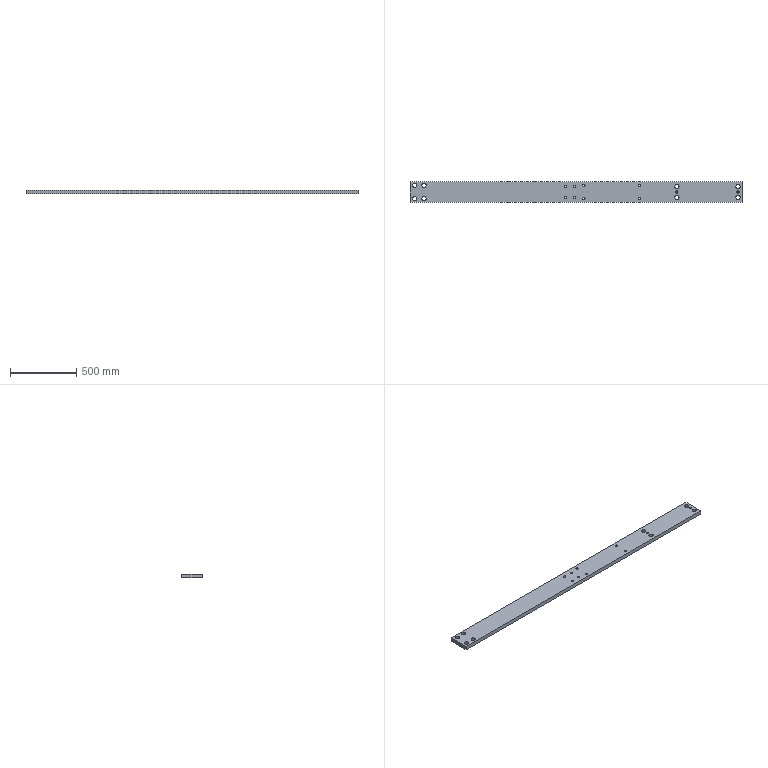Part | NX | features BREP 1 | 1 solid | 42 faces | box 2499 x 158 x 30 mm | volume 11579104 mm3 | cylinder 36 | plane 6 | commonest cylinder face diameters 18 x16 32 x16 16 x4
STEP:
#1=CARTESIAN_POINT('',(-1230.5,-50.,-15.));
#2=VERTEX_POINT('',#1);
#3=CARTESIAN_POINT('',(-1198.5,-50.,-15.));
#4=VERTEX_POINT('',#3);
#5=CARTESIAN_POINT('',(-1214.5,-50.,-15.));
#6=DIRECTION('',(0.,0.,1.));
#7=DIRECTION('',(-1.,0.,0.));
#8=AXIS2_PLACEMENT_3D('',#5,#6,#7);
#9=CIRCLE('',#8,16.);
#10=EDGE_CURVE('',#2,#4,#9,.T.);
#11=ORIENTED_EDGE('',*,*,#10,.F.);
#12=CARTESIAN_POINT('',(-1230.5,-50.,15.));
#13=VERTEX_POINT('',#12);
#14=CARTESIAN_POINT('',(-1230.5,-50.,-15.));
#15=DIRECTION('',(0.,0.,1.));
#16=VECTOR('',#15,1000.);
#17=LINE('',#14,#16);
#18=EDGE_CURVE('',#2,#13,#17,.T.);
#19=ORIENTED_EDGE('',*,*,#18,.T.);
#20=CARTESIAN_POINT('',(-1198.5,-50.,15.));
#21=VERTEX_POINT('',#20);
#22=CARTESIAN_POINT('',(-1214.5,-50.,15.));
#23=DIRECTION('',(0.,0.,1.));
#24=DIRECTION('',(-1.,0.,0.));
#25=AXIS2_PLACEMENT_3D('',#22,#23,#24);
#26=CIRCLE('',#25,16.);
#27=EDGE_CURVE('',#13,#21,#26,.T.);
#28=ORIENTED_EDGE('',*,*,#27,.T.);
#29=CARTESIAN_POINT('',(-1198.5,-50.,-15.));
#30=DIRECTION('',(0.,0.,1.));
#31=VECTOR('',#30,1000.);
#32=LINE('',#29,#31);
#33=EDGE_CURVE('',#4,#21,#32,.T.);
#34=ORIENTED_EDGE('',*,*,#33,.F.);
#35=EDGE_LOOP('',(#11,#19,#28,#34));
#36=FACE_BOUND('',#35,.T.);
#37=CARTESIAN_POINT('',(-1214.5,-50.,-15.));
#38=DIRECTION('',(0.,0.,1.));
#39=DIRECTION('',(-1.,0.,0.));
#40=AXIS2_PLACEMENT_3D('',#37,#38,#39);
#41=CYLINDRICAL_SURFACE('',#40,16.);
#42=ADVANCED_FACE('',(#36),#41,.F.);
#43=CARTESIAN_POINT('',(-1160.5,-50.,-15.));
#44=VERTEX_POINT('',#43);
#45=CARTESIAN_POINT('',(-1128.5,-50.,-15.));
#46=VERTEX_POINT('',#45);
#47=CARTESIAN_POINT('',(-1144.5,-50.,-15.));
#48=DIRECTION('',(0.,0.,1.));
#49=DIRECTION('',(-1.,0.,0.));
#50=AXIS2_PLACEMENT_3D('',#47,#48,#49);
#51=CIRCLE('',#50,16.);
#52=EDGE_CURVE('',#44,#46,#51,.T.);
#53=ORIENTED_EDGE('',*,*,#52,.F.);
#54=CARTESIAN_POINT('',(-1160.5,-50.,15.));
#55=VERTEX_POINT('',#54);
#56=CARTESIAN_POINT('',(-1160.5,-50.,-15.));
#57=DIRECTION('',(0.,0.,1.));
#58=VECTOR('',#57,1000.);
#59=LINE('',#56,#58);
#60=EDGE_CURVE('',#44,#55,#59,.T.);
#61=ORIENTED_EDGE('',*,*,#60,.T.);
#62=CARTESIAN_POINT('',(-1128.5,-50.,15.));
#63=VERTEX_POINT('',#62);
#64=CARTESIAN_POINT('',(-1144.5,-50.,15.));
#65=DIRECTION('',(0.,0.,1.));
#66=DIRECTION('',(-1.,0.,0.));
#67=AXIS2_PLACEMENT_3D('',#64,#65,#66);
#68=CIRCLE('',#67,16.);
#69=EDGE_CURVE('',#55,#63,#68,.T.);
#70=ORIENTED_EDGE('',*,*,#69,.T.);
#71=CARTESIAN_POINT('',(-1128.5,-50.,-15.));
#72=DIRECTION('',(0.,0.,1.));
#73=VECTOR('',#72,1000.);
#74=LINE('',#71,#73);
#75=EDGE_CURVE('',#46,#63,#74,.T.);
#76=ORIENTED_EDGE('',*,*,#75,.F.);
#77=EDGE_LOOP('',(#53,#61,#70,#76));
#78=FACE_BOUND('',#77,.T.);
#79=CARTESIAN_POINT('',(-1144.5,-50.,-15.));
#80=DIRECTION('',(0.,0.,1.));
#81=DIRECTION('',(-1.,0.,0.));
#82=AXIS2_PLACEMENT_3D('',#79,#80,#81);
#83=CYLINDRICAL_SURFACE('',#82,16.);
#84=ADVANCED_FACE('',(#78),#83,.F.);
#85=CARTESIAN_POINT('',(-1160.5,50.,-15.));
#86=VERTEX_POINT('',#85);
#87=CARTESIAN_POINT('',(-1128.5,50.,-15.));
#88=VERTEX_POINT('',#87);
#89=CARTESIAN_POINT('',(-1144.5,50.,-15.));
#90=DIRECTION('',(0.,0.,1.));
#91=DIRECTION('',(1.,0.,0.));
#92=AXIS2_PLACEMENT_3D('',#89,#90,#91);
#93=CIRCLE('',#92,16.);
#94=EDGE_CURVE('',#86,#88,#93,.T.);
#95=ORIENTED_EDGE('',*,*,#94,.F.);
#96=CARTESIAN_POINT('',(-1160.5,50.,15.));
#97=VERTEX_POINT('',#96);
#98=CARTESIAN_POINT('',(-1160.5,50.,-15.));
#99=DIRECTION('',(0.,0.,1.));
#100=VECTOR('',#99,1000.);
#101=LINE('',#98,#100);
#102=EDGE_CURVE('',#86,#97,#101,.T.);
#103=ORIENTED_EDGE('',*,*,#102,.T.);
#104=CARTESIAN_POINT('',(-1128.5,50.,15.));
#105=VERTEX_POINT('',#104);
#106=CARTESIAN_POINT('',(-1144.5,50.,15.));
#107=DIRECTION('',(0.,0.,1.));
#108=DIRECTION('',(1.,0.,0.));
#109=AXIS2_PLACEMENT_3D('',#106,#107,#108);
#110=CIRCLE('',#109,16.);
#111=EDGE_CURVE('',#97,#105,#110,.T.);
#112=ORIENTED_EDGE('',*,*,#111,.T.);
#113=CARTESIAN_POINT('',(-1128.5,50.,-15.));
#114=DIRECTION('',(0.,0.,1.));
#115=VECTOR('',#114,1000.);
#116=LINE('',#113,#115);
#117=EDGE_CURVE('',#88,#105,#116,.T.);
#118=ORIENTED_EDGE('',*,*,#117,.F.);
#119=EDGE_LOOP('',(#95,#103,#112,#118));
#120=FACE_BOUND('',#119,.T.);
#121=CARTESIAN_POINT('',(-1144.5,50.,-15.));
#122=DIRECTION('',(0.,0.,1.));
#123=DIRECTION('',(-1.,0.,0.));
#124=AXIS2_PLACEMENT_3D('',#121,#122,#123);
#125=CYLINDRICAL_SURFACE('',#124,16.);
#126=ADVANCED_FACE('',(#120),#125,.F.);
#127=CARTESIAN_POINT('',(-1230.5,50.,-15.));
#128=VERTEX_POINT('',#127);
#129=CARTESIAN_POINT('',(-1198.5,50.,-15.));
#130=VERTEX_POINT('',#129);
#131=CARTESIAN_POINT('',(-1214.5,50.,-15.));
#132=DIRECTION('',(0.,0.,1.));
#133=DIRECTION('',(1.,0.,0.));
#134=AXIS2_PLACEMENT_3D('',#131,#132,#133);
#135=CIRCLE('',#134,16.);
#136=EDGE_CURVE('',#128,#130,#135,.T.);
#137=ORIENTED_EDGE('',*,*,#136,.F.);
#138=CARTESIAN_POINT('',(-1230.5,50.,15.));
#139=VERTEX_POINT('',#138);
#140=CARTESIAN_POINT('',(-1230.5,50.,-15.));
#141=DIRECTION('',(0.,0.,1.));
#142=VECTOR('',#141,1000.);
#143=LINE('',#140,#142);
#144=EDGE_CURVE('',#128,#139,#143,.T.);
#145=ORIENTED_EDGE('',*,*,#144,.T.);
#146=CARTESIAN_POINT('',(-1198.5,50.,15.));
#147=VERTEX_POINT('',#146);
#148=CARTESIAN_POINT('',(-1214.5,50.,15.));
#149=DIRECTION('',(0.,0.,1.));
#150=DIRECTION('',(1.,0.,0.));
#151=AXIS2_PLACEMENT_3D('',#148,#149,#150);
#152=CIRCLE('',#151,16.);
#153=EDGE_CURVE('',#139,#147,#152,.T.);
#154=ORIENTED_EDGE('',*,*,#153,.T.);
#155=CARTESIAN_POINT('',(-1198.5,50.,-15.));
#156=DIRECTION('',(0.,0.,1.));
#157=VECTOR('',#156,1000.);
#158=LINE('',#155,#157);
#159=EDGE_CURVE('',#130,#147,#158,.T.);
#160=ORIENTED_EDGE('',*,*,#159,.F.);
#161=EDGE_LOOP('',(#137,#145,#154,#160));
#162=FACE_BOUND('',#161,.T.);
#163=CARTESIAN_POINT('',(-1214.5,50.,-15.));
#164=DIRECTION('',(0.,0.,1.));
#165=DIRECTION('',(-1.,0.,0.));
#166=AXIS2_PLACEMENT_3D('',#163,#164,#165);
#167=CYLINDRICAL_SURFACE('',#166,16.);
#168=ADVANCED_FACE('',(#162),#167,.F.);
#169=CARTESIAN_POINT('',(-89.5,-40.,-15.));
#170=VERTEX_POINT('',#169);
#171=CARTESIAN_POINT('',(-71.5,-40.,-15.));
#172=VERTEX_POINT('',#171);
#173=CARTESIAN_POINT('',(-80.5,-40.,-15.));
#174=DIRECTION('',(0.,0.,1.));
#175=DIRECTION('',(1.,0.,0.));
#176=AXIS2_PLACEMENT_3D('',#173,#174,#175);
#177=CIRCLE('',#176,9.);
#178=EDGE_CURVE('',#170,#172,#177,.T.);
#179=ORIENTED_EDGE('',*,*,#178,.F.);
#180=CARTESIAN_POINT('',(-89.5,-40.,15.));
#181=VERTEX_POINT('',#180);
#182=CARTESIAN_POINT('',(-89.5,-40.,-15.));
#183=DIRECTION('',(0.,0.,1.));
#184=VECTOR('',#183,1000.);
#185=LINE('',#182,#184);
#186=EDGE_CURVE('',#170,#181,#185,.T.);
#187=ORIENTED_EDGE('',*,*,#186,.T.);
#188=CARTESIAN_POINT('',(-71.5,-40.,15.));
#189=VERTEX_POINT('',#188);
#190=CARTESIAN_POINT('',(-80.5,-40.,15.));
#191=DIRECTION('',(0.,0.,1.));
#192=DIRECTION('',(1.,0.,0.));
#193=AXIS2_PLACEMENT_3D('',#190,#191,#192);
#194=CIRCLE('',#193,9.);
#195=EDGE_CURVE('',#181,#189,#194,.T.);
#196=ORIENTED_EDGE('',*,*,#195,.T.);
#197=CARTESIAN_POINT('',(-71.5,-40.,-15.));
#198=DIRECTION('',(0.,0.,1.));
#199=VECTOR('',#198,1000.);
#200=LINE('',#197,#199);
#201=EDGE_CURVE('',#172,#189,#200,.T.);
#202=ORIENTED_EDGE('',*,*,#201,.F.);
#203=EDGE_LOOP('',(#179,#187,#196,#202));
#204=FACE_BOUND('',#203,.T.);
#205=CARTESIAN_POINT('',(-80.5,-40.,-15.));
#206=DIRECTION('',(0.,0.,1.));
#207=DIRECTION('',(-1.,0.,0.));
#208=AXIS2_PLACEMENT_3D('',#205,#206,#207);
#209=CYLINDRICAL_SURFACE('',#208,9.);
#210=ADVANCED_FACE('',(#204),#209,.F.);
#211=CARTESIAN_POINT('',(-19.5,-40.,-15.));
#212=VERTEX_POINT('',#211);
#213=CARTESIAN_POINT('',(-1.5,-40.,-15.));
#214=VERTEX_POINT('',#213);
#215=CARTESIAN_POINT('',(-10.5,-40.,-15.));
#216=DIRECTION('',(0.,0.,1.));
#217=DIRECTION('',(1.,0.,0.));
#218=AXIS2_PLACEMENT_3D('',#215,#216,#217);
#219=CIRCLE('',#218,9.);
#220=EDGE_CURVE('',#212,#214,#219,.T.);
#221=ORIENTED_EDGE('',*,*,#220,.F.);
#222=CARTESIAN_POINT('',(-19.5,-40.,15.));
#223=VERTEX_POINT('',#222);
#224=CARTESIAN_POINT('',(-19.5,-40.,-15.));
#225=DIRECTION('',(0.,0.,1.));
#226=VECTOR('',#225,1000.);
#227=LINE('',#224,#226);
#228=EDGE_CURVE('',#212,#223,#227,.T.);
#229=ORIENTED_EDGE('',*,*,#228,.T.);
#230=CARTESIAN_POINT('',(-1.5,-40.,15.));
#231=VERTEX_POINT('',#230);
#232=CARTESIAN_POINT('',(-10.5,-40.,15.));
#233=DIRECTION('',(0.,0.,1.));
#234=DIRECTION('',(1.,0.,0.));
#235=AXIS2_PLACEMENT_3D('',#232,#233,#234);
#236=CIRCLE('',#235,9.);
#237=EDGE_CURVE('',#223,#231,#236,.T.);
#238=ORIENTED_EDGE('',*,*,#237,.T.);
#239=CARTESIAN_POINT('',(-1.5,-40.,-15.));
#240=DIRECTION('',(0.,0.,1.));
#241=VECTOR('',#240,1000.);
#242=LINE('',#239,#241);
#243=EDGE_CURVE('',#214,#231,#242,.T.);
#244=ORIENTED_EDGE('',*,*,#243,.F.);
#245=EDGE_LOOP('',(#221,#229,#238,#244));
#246=FACE_BOUND('',#245,.T.);
#247=CARTESIAN_POINT('',(-10.5,-40.,-15.));
#248=DIRECTION('',(0.,0.,1.));
#249=DIRECTION('',(-1.,0.,0.));
#250=AXIS2_PLACEMENT_3D('',#247,#248,#249);
#251=CYLINDRICAL_SURFACE('',#250,9.);
#252=ADVANCED_FACE('',(#246),#251,.F.);
#253=CARTESIAN_POINT('',(-89.5,40.,-15.));
#254=VERTEX_POINT('',#253);
#255=CARTESIAN_POINT('',(-71.5,40.,-15.));
#256=VERTEX_POINT('',#255);
#257=CARTESIAN_POINT('',(-80.5,40.,-15.));
#258=DIRECTION('',(0.,0.,1.));
#259=DIRECTION('',(1.,0.,0.));
#260=AXIS2_PLACEMENT_3D('',#257,#258,#259);
#261=CIRCLE('',#260,9.);
#262=EDGE_CURVE('',#254,#256,#261,.T.);
#263=ORIENTED_EDGE('',*,*,#262,.F.);
#264=CARTESIAN_POINT('',(-89.5,40.,15.));
#265=VERTEX_POINT('',#264);
#266=CARTESIAN_POINT('',(-89.5,40.,-15.));
#267=DIRECTION('',(0.,0.,1.));
#268=VECTOR('',#267,1000.);
#269=LINE('',#266,#268);
#270=EDGE_CURVE('',#254,#265,#269,.T.);
#271=ORIENTED_EDGE('',*,*,#270,.T.);
#272=CARTESIAN_POINT('',(-71.5,40.,15.));
#273=VERTEX_POINT('',#272);
#274=CARTESIAN_POINT('',(-80.5,40.,15.));
#275=DIRECTION('',(0.,0.,1.));
#276=DIRECTION('',(1.,0.,0.));
#277=AXIS2_PLACEMENT_3D('',#274,#275,#276);
#278=CIRCLE('',#277,9.);
#279=EDGE_CURVE('',#265,#273,#278,.T.);
#280=ORIENTED_EDGE('',*,*,#279,.T.);
#281=CARTESIAN_POINT('',(-71.5,40.,-15.));
#282=DIRECTION('',(0.,0.,1.));
#283=VECTOR('',#282,1000.);
#284=LINE('',#281,#283);
#285=EDGE_CURVE('',#256,#273,#284,.T.);
#286=ORIENTED_EDGE('',*,*,#285,.F.);
#287=EDGE_LOOP('',(#263,#271,#280,#286));
#288=FACE_BOUND('',#287,.T.);
#289=CARTESIAN_POINT('',(-80.5,40.,-15.));
#290=DIRECTION('',(0.,0.,1.));
#291=DIRECTION('',(-1.,0.,0.));
#292=AXIS2_PLACEMENT_3D('',#289,#290,#291);
#293=CYLINDRICAL_SURFACE('',#292,9.);
#294=ADVANCED_FACE('',(#288),#293,.F.);
#295=CARTESIAN_POINT('',(-19.5,40.,-15.));
#296=VERTEX_POINT('',#295);
#297=CARTESIAN_POINT('',(-1.5,40.,-15.));
#298=VERTEX_POINT('',#297);
#299=CARTESIAN_POINT('',(-10.5,40.,-15.));
#300=DIRECTION('',(0.,0.,1.));
#301=DIRECTION('',(1.,0.,0.));
#302=AXIS2_PLACEMENT_3D('',#299,#300,#301);
#303=CIRCLE('',#302,9.);
#304=EDGE_CURVE('',#296,#298,#303,.T.);
#305=ORIENTED_EDGE('',*,*,#304,.F.);
#306=CARTESIAN_POINT('',(-19.5,40.,15.));
#307=VERTEX_POINT('',#306);
#308=CARTESIAN_POINT('',(-19.5,40.,-15.));
#309=DIRECTION('',(0.,0.,1.));
#310=VECTOR('',#309,1000.);
#311=LINE('',#308,#310);
#312=EDGE_CURVE('',#296,#307,#311,.T.);
#313=ORIENTED_EDGE('',*,*,#312,.T.);
#314=CARTESIAN_POINT('',(-1.5,40.,15.));
#315=VERTEX_POINT('',#314);
#316=CARTESIAN_POINT('',(-10.5,40.,15.));
#317=DIRECTION('',(0.,0.,1.));
#318=DIRECTION('',(1.,0.,0.));
#319=AXIS2_PLACEMENT_3D('',#316,#317,#318);
#320=CIRCLE('',#319,9.);
#321=EDGE_CURVE('',#307,#315,#320,.T.);
#322=ORIENTED_EDGE('',*,*,#321,.T.);
#323=CARTESIAN_POINT('',(-1.5,40.,-15.));
#324=DIRECTION('',(0.,0.,1.));
#325=VECTOR('',#324,1000.);
#326=LINE('',#323,#325);
#327=EDGE_CURVE('',#298,#315,#326,.T.);
#328=ORIENTED_EDGE('',*,*,#327,.F.);
#329=EDGE_LOOP('',(#305,#313,#322,#328));
#330=FACE_BOUND('',#329,.T.);
#331=CARTESIAN_POINT('',(-10.5,40.,-15.));
#332=DIRECTION('',(0.,0.,1.));
#333=DIRECTION('',(-1.,0.,0.));
#334=AXIS2_PLACEMENT_3D('',#331,#332,#333);
#335=CYLINDRICAL_SURFACE('',#334,9.);
#336=ADVANCED_FACE('',(#330),#335,.F.);
#337=CARTESIAN_POINT('',(50.5,-50.,-15.));
#338=VERTEX_POINT('',#337);
#339=CARTESIAN_POINT('',(68.5,-50.,-15.));
#340=VERTEX_POINT('',#339);
#341=CARTESIAN_POINT('',(59.5,-50.,-15.));
#342=DIRECTION('',(0.,0.,1.));
#343=DIRECTION('',(1.,0.,0.));
#344=AXIS2_PLACEMENT_3D('',#341,#342,#343);
#345=CIRCLE('',#344,9.);
#346=EDGE_CURVE('',#338,#340,#345,.T.);
#347=ORIENTED_EDGE('',*,*,#346,.F.);
#348=CARTESIAN_POINT('',(50.5,-50.,15.));
#349=VERTEX_POINT('',#348);
#350=CARTESIAN_POINT('',(50.5,-50.,-15.));
#351=DIRECTION('',(0.,0.,1.));
#352=VECTOR('',#351,1000.);
#353=LINE('',#350,#352);
#354=EDGE_CURVE('',#338,#349,#353,.T.);
#355=ORIENTED_EDGE('',*,*,#354,.T.);
#356=CARTESIAN_POINT('',(68.5,-50.,15.));
#357=VERTEX_POINT('',#356);
#358=CARTESIAN_POINT('',(59.5,-50.,15.));
#359=DIRECTION('',(0.,0.,1.));
#360=DIRECTION('',(1.,0.,0.));
#361=AXIS2_PLACEMENT_3D('',#358,#359,#360);
#362=CIRCLE('',#361,9.);
#363=EDGE_CURVE('',#349,#357,#362,.T.);
#364=ORIENTED_EDGE('',*,*,#363,.T.);
#365=CARTESIAN_POINT('',(68.5,-50.,-15.));
#366=DIRECTION('',(0.,0.,1.));
#367=VECTOR('',#366,1000.);
#368=LINE('',#365,#367);
#369=EDGE_CURVE('',#340,#357,#368,.T.);
#370=ORIENTED_EDGE('',*,*,#369,.F.);
#371=EDGE_LOOP('',(#347,#355,#364,#370));
#372=FACE_BOUND('',#371,.T.);
#373=CARTESIAN_POINT('',(59.5,-50.,-15.));
#374=DIRECTION('',(0.,0.,1.));
#375=DIRECTION('',(-1.,0.,0.));
#376=AXIS2_PLACEMENT_3D('',#373,#374,#375);
#377=CYLINDRICAL_SURFACE('',#376,9.);
#378=ADVANCED_FACE('',(#372),#377,.F.);
#379=CARTESIAN_POINT('',(50.5,50.,-15.));
#380=VERTEX_POINT('',#379);
#381=CARTESIAN_POINT('',(68.5,50.,-15.));
#382=VERTEX_POINT('',#381);
#383=CARTESIAN_POINT('',(59.5,50.,-15.));
#384=DIRECTION('',(0.,0.,1.));
#385=DIRECTION('',(-1.,0.,0.));
#386=AXIS2_PLACEMENT_3D('',#383,#384,#385);
#387=CIRCLE('',#386,9.);
#388=EDGE_CURVE('',#380,#382,#387,.T.);
#389=ORIENTED_EDGE('',*,*,#388,.F.);
#390=CARTESIAN_POINT('',(50.5,50.,15.));
#391=VERTEX_POINT('',#390);
#392=CARTESIAN_POINT('',(50.5,50.,-15.));
#393=DIRECTION('',(0.,0.,1.));
#394=VECTOR('',#393,1000.);
#395=LINE('',#392,#394);
#396=EDGE_CURVE('',#380,#391,#395,.T.);
#397=ORIENTED_EDGE('',*,*,#396,.T.);
#398=CARTESIAN_POINT('',(68.5,50.,15.));
#399=VERTEX_POINT('',#398);
#400=CARTESIAN_POINT('',(59.5,50.,15.));
#401=DIRECTION('',(0.,0.,1.));
#402=DIRECTION('',(-1.,0.,0.));
#403=AXIS2_PLACEMENT_3D('',#400,#401,#402);
#404=CIRCLE('',#403,9.);
#405=EDGE_CURVE('',#391,#399,#404,.T.);
#406=ORIENTED_EDGE('',*,*,#405,.T.);
#407=CARTESIAN_POINT('',(68.5,50.,-15.));
#408=DIRECTION('',(0.,0.,1.));
#409=VECTOR('',#408,1000.);
#410=LINE('',#407,#409);
#411=EDGE_CURVE('',#382,#399,#410,.T.);
#412=ORIENTED_EDGE('',*,*,#411,.F.);
#413=EDGE_LOOP('',(#389,#397,#406,#412));
#414=FACE_BOUND('',#413,.T.);
#415=CARTESIAN_POINT('',(59.5,50.,-15.));
#416=DIRECTION('',(0.,0.,1.));
#417=DIRECTION('',(-1.,0.,0.));
#418=AXIS2_PLACEMENT_3D('',#415,#416,#417);
#419=CYLINDRICAL_SURFACE('',#418,9.);
#420=ADVANCED_FACE('',(#414),#419,.F.);
#421=CARTESIAN_POINT('',(470.5,-50.,-15.));
#422=VERTEX_POINT('',#421);
#423=CARTESIAN_POINT('',(488.5,-50.,-15.));
#424=VERTEX_POINT('',#423);
#425=CARTESIAN_POINT('',(479.5,-50.,-15.));
#426=DIRECTION('',(0.,0.,1.));
#427=DIRECTION('',(-1.,0.,0.));
#428=AXIS2_PLACEMENT_3D('',#425,#426,#427);
#429=CIRCLE('',#428,9.);
#430=EDGE_CURVE('',#422,#424,#429,.T.);
#431=ORIENTED_EDGE('',*,*,#430,.F.);
#432=CARTESIAN_POINT('',(470.5,-50.,15.));
#433=VERTEX_POINT('',#432);
#434=CARTESIAN_POINT('',(470.5,-50.,-15.));
#435=DIRECTION('',(0.,0.,1.));
#436=VECTOR('',#435,1000.);
#437=LINE('',#434,#436);
#438=EDGE_CURVE('',#422,#433,#437,.T.);
#439=ORIENTED_EDGE('',*,*,#438,.T.);
#440=CARTESIAN_POINT('',(488.5,-50.,15.));
#441=VERTEX_POINT('',#440);
#442=CARTESIAN_POINT('',(479.5,-50.,15.));
#443=DIRECTION('',(0.,0.,1.));
#444=DIRECTION('',(-1.,0.,0.));
#445=AXIS2_PLACEMENT_3D('',#442,#443,#444);
#446=CIRCLE('',#445,9.);
#447=EDGE_CURVE('',#433,#441,#446,.T.);
#448=ORIENTED_EDGE('',*,*,#447,.T.);
#449=CARTESIAN_POINT('',(488.5,-50.,-15.));
#450=DIRECTION('',(0.,0.,1.));
#451=VECTOR('',#450,1000.);
#452=LINE('',#449,#451);
#453=EDGE_CURVE('',#424,#441,#452,.T.);
#454=ORIENTED_EDGE('',*,*,#453,.F.);
#455=EDGE_LOOP('',(#431,#439,#448,#454));
#456=FACE_BOUND('',#455,.T.);
#457=CARTESIAN_POINT('',(479.5,-50.,-15.));
#458=DIRECTION('',(0.,0.,1.));
#459=DIRECTION('',(-1.,0.,0.));
#460=AXIS2_PLACEMENT_3D('',#457,#458,#459);
#461=CYLINDRICAL_SURFACE('',#460,9.);
#462=ADVANCED_FACE('',(#456),#461,.F.);
#463=CARTESIAN_POINT('',(470.5,50.,-15.));
#464=VERTEX_POINT('',#463);
#465=CARTESIAN_POINT('',(488.5,50.,-15.));
#466=VERTEX_POINT('',#465);
#467=CARTESIAN_POINT('',(479.5,50.,-15.));
#468=DIRECTION('',(0.,0.,1.));
#469=DIRECTION('',(1.,0.,0.));
#470=AXIS2_PLACEMENT_3D('',#467,#468,#469);
#471=CIRCLE('',#470,9.);
#472=EDGE_CURVE('',#464,#466,#471,.T.);
#473=ORIENTED_EDGE('',*,*,#472,.F.);
#474=CARTESIAN_POINT('',(470.5,50.,15.));
#475=VERTEX_POINT('',#474);
#476=CARTESIAN_POINT('',(470.5,50.,-15.));
#477=DIRECTION('',(0.,0.,1.));
#478=VECTOR('',#477,1000.);
#479=LINE('',#476,#478);
#480=EDGE_CURVE('',#464,#475,#479,.T.);
#481=ORIENTED_EDGE('',*,*,#480,.T.);
#482=CARTESIAN_POINT('',(488.5,50.,15.));
#483=VERTEX_POINT('',#482);
#484=CARTESIAN_POINT('',(479.5,50.,15.));
#485=DIRECTION('',(0.,0.,1.));
#486=DIRECTION('',(1.,0.,0.));
#487=AXIS2_PLACEMENT_3D('',#484,#485,#486);
#488=CIRCLE('',#487,9.);
#489=EDGE_CURVE('',#475,#483,#488,.T.);
#490=ORIENTED_EDGE('',*,*,#489,.T.);
#491=CARTESIAN_POINT('',(488.5,50.,-15.));
#492=DIRECTION('',(0.,0.,1.));
#493=VECTOR('',#492,1000.);
#494=LINE('',#491,#493);
#495=EDGE_CURVE('',#466,#483,#494,.T.);
#496=ORIENTED_EDGE('',*,*,#495,.F.);
#497=EDGE_LOOP('',(#473,#481,#490,#496));
#498=FACE_BOUND('',#497,.T.);
#499=CARTESIAN_POINT('',(479.5,50.,-15.));
#500=DIRECTION('',(0.,0.,1.));
#501=DIRECTION('',(-1.,0.,0.));
#502=AXIS2_PLACEMENT_3D('',#499,#500,#501);
#503=CYLINDRICAL_SURFACE('',#502,9.);
#504=ADVANCED_FACE('',(#498),#503,.F.);
#505=CARTESIAN_POINT('',(743.5,40.,-15.));
#506=VERTEX_POINT('',#505);
#507=CARTESIAN_POINT('',(775.5,40.,-15.));
#508=VERTEX_POINT('',#507);
#509=CARTESIAN_POINT('',(759.5,40.,-15.));
#510=DIRECTION('',(0.,0.,1.));
#511=DIRECTION('',(-1.,0.,0.));
#512=AXIS2_PLACEMENT_3D('',#509,#510,#511);
#513=CIRCLE('',#512,16.);
#514=EDGE_CURVE('',#506,#508,#513,.T.);
#515=ORIENTED_EDGE('',*,*,#514,.F.);
#516=CARTESIAN_POINT('',(743.5,40.,15.));
#517=VERTEX_POINT('',#516);
#518=CARTESIAN_POINT('',(743.5,40.,-15.));
#519=DIRECTION('',(0.,0.,1.));
#520=VECTOR('',#519,1000.);
#521=LINE('',#518,#520);
#522=EDGE_CURVE('',#506,#517,#521,.T.);
#523=ORIENTED_EDGE('',*,*,#522,.T.);
#524=CARTESIAN_POINT('',(775.5,40.,15.));
#525=VERTEX_POINT('',#524);
#526=CARTESIAN_POINT('',(759.5,40.,15.));
#527=DIRECTION('',(0.,0.,1.));
#528=DIRECTION('',(-1.,0.,0.));
#529=AXIS2_PLACEMENT_3D('',#526,#527,#528);
#530=CIRCLE('',#529,16.);
#531=EDGE_CURVE('',#517,#525,#530,.T.);
#532=ORIENTED_EDGE('',*,*,#531,.T.);
#533=CARTESIAN_POINT('',(775.5,40.,-15.));
#534=DIRECTION('',(0.,0.,1.));
#535=VECTOR('',#534,1000.);
#536=LINE('',#533,#535);
#537=EDGE_CURVE('',#508,#525,#536,.T.);
#538=ORIENTED_EDGE('',*,*,#537,.F.);
#539=EDGE_LOOP('',(#515,#523,#532,#538));
#540=FACE_BOUND('',#539,.T.);
#541=CARTESIAN_POINT('',(759.5,40.,-15.));
#542=DIRECTION('',(0.,0.,1.));
#543=DIRECTION('',(-1.,0.,0.));
#544=AXIS2_PLACEMENT_3D('',#541,#542,#543);
#545=CYLINDRICAL_SURFACE('',#544,16.);
#546=ADVANCED_FACE('',(#540),#545,.F.);
#547=CARTESIAN_POINT('',(743.5,-40.,-15.));
#548=VERTEX_POINT('',#547);
#549=CARTESIAN_POINT('',(775.5,-40.,-15.));
#550=VERTEX_POINT('',#549);
#551=CARTESIAN_POINT('',(759.5,-40.,-15.));
#552=DIRECTION('',(0.,0.,1.));
#553=DIRECTION('',(1.,0.,0.));
#554=AXIS2_PLACEMENT_3D('',#551,#552,#553);
#555=CIRCLE('',#554,16.);
#556=EDGE_CURVE('',#548,#550,#555,.T.);
#557=ORIENTED_EDGE('',*,*,#556,.F.);
#558=CARTESIAN_POINT('',(743.5,-40.,15.));
#559=VERTEX_POINT('',#558);
#560=CARTESIAN_POINT('',(743.5,-40.,-15.));
#561=DIRECTION('',(0.,0.,1.));
#562=VECTOR('',#561,1000.);
#563=LINE('',#560,#562);
#564=EDGE_CURVE('',#548,#559,#563,.T.);
#565=ORIENTED_EDGE('',*,*,#564,.T.);
#566=CARTESIAN_POINT('',(775.5,-40.,15.));
#567=VERTEX_POINT('',#566);
#568=CARTESIAN_POINT('',(759.5,-40.,15.));
#569=DIRECTION('',(0.,0.,1.));
#570=DIRECTION('',(1.,0.,0.));
#571=AXIS2_PLACEMENT_3D('',#568,#569,#570);
#572=CIRCLE('',#571,16.);
#573=EDGE_CURVE('',#559,#567,#572,.T.);
#574=ORIENTED_EDGE('',*,*,#573,.T.);
#575=CARTESIAN_POINT('',(775.5,-40.,-15.));
#576=DIRECTION('',(0.,0.,1.));
#577=VECTOR('',#576,1000.);
#578=LINE('',#575,#577);
#579=EDGE_CURVE('',#550,#567,#578,.T.);
#580=ORIENTED_EDGE('',*,*,#579,.F.);
#581=EDGE_LOOP('',(#557,#565,#574,#580));
#582=FACE_BOUND('',#581,.T.);
#583=CARTESIAN_POINT('',(759.5,-40.,-15.));
#584=DIRECTION('',(0.,0.,1.));
#585=DIRECTION('',(-1.,0.,0.));
#586=AXIS2_PLACEMENT_3D('',#583,#584,#585);
#587=CYLINDRICAL_SURFACE('',#586,16.);
#588=ADVANCED_FACE('',(#582),#587,.F.);
#589=CARTESIAN_POINT('',(751.5,0.,-15.));
#590=VERTEX_POINT('',#589);
#591=CARTESIAN_POINT('',(767.5,0.,-15.));
#592=VERTEX_POINT('',#591);
#593=CARTESIAN_POINT('',(759.5,0.,-15.));
#594=DIRECTION('',(0.,0.,1.));
#595=DIRECTION('',(-1.,0.,0.));
#596=AXIS2_PLACEMENT_3D('',#593,#594,#595);
#597=CIRCLE('',#596,8.);
#598=EDGE_CURVE('',#590,#592,#597,.T.);
#599=ORIENTED_EDGE('',*,*,#598,.F.);
#600=CARTESIAN_POINT('',(751.5,0.,15.));
#601=VERTEX_POINT('',#600);
#602=CARTESIAN_POINT('',(751.5,0.,-15.));
#603=DIRECTION('',(0.,0.,1.));
#604=VECTOR('',#603,1000.);
#605=LINE('',#602,#604);
#606=EDGE_CURVE('',#590,#601,#605,.T.);
#607=ORIENTED_EDGE('',*,*,#606,.T.);
#608=CARTESIAN_POINT('',(767.5,0.,15.));
#609=VERTEX_POINT('',#608);
#610=CARTESIAN_POINT('',(759.5,0.,15.));
#611=DIRECTION('',(0.,0.,1.));
#612=DIRECTION('',(-1.,0.,0.));
#613=AXIS2_PLACEMENT_3D('',#610,#611,#612);
#614=CIRCLE('',#613,8.);
#615=EDGE_CURVE('',#601,#609,#614,.T.);
#616=ORIENTED_EDGE('',*,*,#615,.T.);
#617=CARTESIAN_POINT('',(767.5,0.,-15.));
#618=DIRECTION('',(0.,0.,1.));
#619=VECTOR('',#618,1000.);
#620=LINE('',#617,#619);
#621=EDGE_CURVE('',#592,#609,#620,.T.);
#622=ORIENTED_EDGE('',*,*,#621,.F.);
#623=EDGE_LOOP('',(#599,#607,#616,#622));
#624=FACE_BOUND('',#623,.T.);
#625=CARTESIAN_POINT('',(759.5,0.,-15.));
#626=DIRECTION('',(0.,0.,1.));
#627=DIRECTION('',(-1.,0.,0.));
#628=AXIS2_PLACEMENT_3D('',#625,#626,#627);
#629=CYLINDRICAL_SURFACE('',#628,8.);
#630=ADVANCED_FACE('',(#624),#629,.F.);
#631=CARTESIAN_POINT('',(1211.5,0.,-15.));
#632=VERTEX_POINT('',#631);
#633=CARTESIAN_POINT('',(1227.5,0.,-15.));
#634=VERTEX_POINT('',#633);
#635=CARTESIAN_POINT('',(1219.5,0.,-15.));
#636=DIRECTION('',(0.,0.,1.));
#637=DIRECTION('',(1.,0.,0.));
#638=AXIS2_PLACEMENT_3D('',#635,#636,#637);
#639=CIRCLE('',#638,8.);
#640=EDGE_CURVE('',#632,#634,#639,.T.);
#641=ORIENTED_EDGE('',*,*,#640,.F.);
#642=CARTESIAN_POINT('',(1211.5,0.,15.));
#643=VERTEX_POINT('',#642);
#644=CARTESIAN_POINT('',(1211.5,0.,-15.));
#645=DIRECTION('',(0.,0.,1.));
#646=VECTOR('',#645,1000.);
#647=LINE('',#644,#646);
#648=EDGE_CURVE('',#632,#643,#647,.T.);
#649=ORIENTED_EDGE('',*,*,#648,.T.);
#650=CARTESIAN_POINT('',(1227.5,0.,15.));
#651=VERTEX_POINT('',#650);
#652=CARTESIAN_POINT('',(1219.5,0.,15.));
#653=DIRECTION('',(0.,0.,1.));
#654=DIRECTION('',(1.,0.,0.));
#655=AXIS2_PLACEMENT_3D('',#652,#653,#654);
#656=CIRCLE('',#655,8.);
#657=EDGE_CURVE('',#643,#651,#656,.T.);
#658=ORIENTED_EDGE('',*,*,#657,.T.);
#659=CARTESIAN_POINT('',(1227.5,0.,-15.));
#660=DIRECTION('',(0.,0.,1.));
#661=VECTOR('',#660,1000.);
#662=LINE('',#659,#661);
#663=EDGE_CURVE('',#634,#651,#662,.T.);
#664=ORIENTED_EDGE('',*,*,#663,.F.);
#665=EDGE_LOOP('',(#641,#649,#658,#664));
#666=FACE_BOUND('',#665,.T.);
#667=CARTESIAN_POINT('',(1219.5,0.,-15.));
#668=DIRECTION('',(0.,0.,1.));
#669=DIRECTION('',(-1.,0.,0.));
#670=AXIS2_PLACEMENT_3D('',#667,#668,#669);
#671=CYLINDRICAL_SURFACE('',#670,8.);
#672=ADVANCED_FACE('',(#666),#671,.F.);
#673=CARTESIAN_POINT('',(1203.5,-40.,-15.));
#674=VERTEX_POINT('',#673);
#675=CARTESIAN_POINT('',(1235.5,-40.,-15.));
#676=VERTEX_POINT('',#675);
#677=CARTESIAN_POINT('',(1219.5,-40.,-15.));
#678=DIRECTION('',(0.,0.,1.));
#679=DIRECTION('',(-1.,0.,0.));
#680=AXIS2_PLACEMENT_3D('',#677,#678,#679);
#681=CIRCLE('',#680,16.);
#682=EDGE_CURVE('',#674,#676,#681,.T.);
#683=ORIENTED_EDGE('',*,*,#682,.F.);
#684=CARTESIAN_POINT('',(1203.5,-40.,15.));
#685=VERTEX_POINT('',#684);
#686=CARTESIAN_POINT('',(1203.5,-40.,-15.));
#687=DIRECTION('',(0.,0.,1.));
#688=VECTOR('',#687,1000.);
#689=LINE('',#686,#688);
#690=EDGE_CURVE('',#674,#685,#689,.T.);
#691=ORIENTED_EDGE('',*,*,#690,.T.);
#692=CARTESIAN_POINT('',(1235.5,-40.,15.));
#693=VERTEX_POINT('',#692);
#694=CARTESIAN_POINT('',(1219.5,-40.,15.));
#695=DIRECTION('',(0.,0.,1.));
#696=DIRECTION('',(-1.,0.,0.));
#697=AXIS2_PLACEMENT_3D('',#694,#695,#696);
#698=CIRCLE('',#697,16.);
#699=EDGE_CURVE('',#685,#693,#698,.T.);
#700=ORIENTED_EDGE('',*,*,#699,.T.);
#701=CARTESIAN_POINT('',(1235.5,-40.,-15.));
#702=DIRECTION('',(0.,0.,1.));
#703=VECTOR('',#702,1000.);
#704=LINE('',#701,#703);
#705=EDGE_CURVE('',#676,#693,#704,.T.);
#706=ORIENTED_EDGE('',*,*,#705,.F.);
#707=EDGE_LOOP('',(#683,#691,#700,#706));
#708=FACE_BOUND('',#707,.T.);
#709=CARTESIAN_POINT('',(1219.5,-40.,-15.));
#710=DIRECTION('',(0.,0.,1.));
#711=DIRECTION('',(-1.,0.,0.));
#712=AXIS2_PLACEMENT_3D('',#709,#710,#711);
#713=CYLINDRICAL_SURFACE('',#712,16.);
#714=ADVANCED_FACE('',(#708),#713,.F.);
#715=CARTESIAN_POINT('',(1203.5,40.,-15.));
#716=VERTEX_POINT('',#715);
#717=CARTESIAN_POINT('',(1235.5,40.,-15.));
#718=VERTEX_POINT('',#717);
#719=CARTESIAN_POINT('',(1219.5,40.,-15.));
#720=DIRECTION('',(0.,0.,1.));
#721=DIRECTION('',(1.,0.,0.));
#722=AXIS2_PLACEMENT_3D('',#719,#720,#721);
#723=CIRCLE('',#722,16.);
#724=EDGE_CURVE('',#716,#718,#723,.T.);
#725=ORIENTED_EDGE('',*,*,#724,.F.);
#726=CARTESIAN_POINT('',(1203.5,40.,15.));
#727=VERTEX_POINT('',#726);
#728=CARTESIAN_POINT('',(1203.5,40.,-15.));
#729=DIRECTION('',(0.,0.,1.));
#730=VECTOR('',#729,1000.);
#731=LINE('',#728,#730);
#732=EDGE_CURVE('',#716,#727,#731,.T.);
#733=ORIENTED_EDGE('',*,*,#732,.T.);
#734=CARTESIAN_POINT('',(1235.5,40.,15.));
#735=VERTEX_POINT('',#734);
#736=CARTESIAN_POINT('',(1219.5,40.,15.));
#737=DIRECTION('',(0.,0.,1.));
#738=DIRECTION('',(1.,0.,0.));
#739=AXIS2_PLACEMENT_3D('',#736,#737,#738);
#740=CIRCLE('',#739,16.);
#741=EDGE_CURVE('',#727,#735,#740,.T.);
#742=ORIENTED_EDGE('',*,*,#741,.T.);
#743=CARTESIAN_POINT('',(1235.5,40.,-15.));
#744=DIRECTION('',(0.,0.,1.));
#745=VECTOR('',#744,1000.);
#746=LINE('',#743,#745);
#747=EDGE_CURVE('',#718,#735,#746,.T.);
#748=ORIENTED_EDGE('',*,*,#747,.F.);
#749=EDGE_LOOP('',(#725,#733,#742,#748));
#750=FACE_BOUND('',#749,.T.);
#751=CARTESIAN_POINT('',(1219.5,40.,-15.));
#752=DIRECTION('',(0.,0.,1.));
#753=DIRECTION('',(-1.,0.,0.));
#754=AXIS2_PLACEMENT_3D('',#751,#752,#753);
#755=CYLINDRICAL_SURFACE('',#754,16.);
#756=ADVANCED_FACE('',(#750),#755,.F.);
#757=CARTESIAN_POINT('',(-1249.5,79.,-15.));
#758=VERTEX_POINT('',#757);
#759=CARTESIAN_POINT('',(-1249.5,-79.,-15.));
#760=VERTEX_POINT('',#759);
#761=CARTESIAN_POINT('',(-1249.5,79.,-15.));
#762=DIRECTION('',(0.,-1.,0.));
#763=VECTOR('',#762,1000.);
#764=LINE('',#761,#763);
#765=EDGE_CURVE('',#758,#760,#764,.T.);
#766=ORIENTED_EDGE('',*,*,#765,.T.);
#767=CARTESIAN_POINT('',(-1249.5,-79.,15.));
#768=VERTEX_POINT('',#767);
#769=CARTESIAN_POINT('',(-1249.5,-79.,15.));
#770=DIRECTION('',(0.,0.,-1.));
#771=VECTOR('',#770,1000.);
#772=LINE('',#769,#771);
#773=EDGE_CURVE('',#768,#760,#772,.T.);
#774=ORIENTED_EDGE('',*,*,#773,.F.);
#775=CARTESIAN_POINT('',(-1249.5,79.,15.));
#776=VERTEX_POINT('',#775);
#777=CARTESIAN_POINT('',(-1249.5,79.,15.));
#778=DIRECTION('',(0.,-1.,0.));
#779=VECTOR('',#778,1000.);
#780=LINE('',#777,#779);
#781=EDGE_CURVE('',#776,#768,#780,.T.);
#782=ORIENTED_EDGE('',*,*,#781,.F.);
#783=CARTESIAN_POINT('',(-1249.5,79.,15.));
#784=DIRECTION('',(0.,0.,-1.));
#785=VECTOR('',#784,1000.);
#786=LINE('',#783,#785);
#787=EDGE_CURVE('',#776,#758,#786,.T.);
#788=ORIENTED_EDGE('',*,*,#787,.T.);
#789=EDGE_LOOP('',(#766,#774,#782,#788));
#790=FACE_BOUND('',#789,.T.);
#791=CARTESIAN_POINT('',(-1249.5,79.,15.));
#792=DIRECTION('',(1.,0.,0.));
#793=DIRECTION('',(0.,0.,1.));
#794=AXIS2_PLACEMENT_3D('',#791,#792,#793);
#795=PLANE('',#794);
#796=ADVANCED_FACE('',(#790),#795,.F.);
#797=CARTESIAN_POINT('',(1249.5,-79.,-15.));
#798=VERTEX_POINT('',#797);
#799=CARTESIAN_POINT('',(-1249.5,-79.,-15.));
#800=DIRECTION('',(1.,0.,0.));
#801=VECTOR('',#800,1000.);
#802=LINE('',#799,#801);
#803=EDGE_CURVE('',#760,#798,#802,.T.);
#804=ORIENTED_EDGE('',*,*,#803,.T.);
#805=CARTESIAN_POINT('',(1249.5,-79.,15.));
#806=VERTEX_POINT('',#805);
#807=CARTESIAN_POINT('',(1249.5,-79.,15.));
#808=DIRECTION('',(0.,0.,-1.));
#809=VECTOR('',#808,1000.);
#810=LINE('',#807,#809);
#811=EDGE_CURVE('',#806,#798,#810,.T.);
#812=ORIENTED_EDGE('',*,*,#811,.F.);
#813=CARTESIAN_POINT('',(-1249.5,-79.,15.));
#814=DIRECTION('',(1.,0.,0.));
#815=VECTOR('',#814,1000.);
#816=LINE('',#813,#815);
#817=EDGE_CURVE('',#768,#806,#816,.T.);
#818=ORIENTED_EDGE('',*,*,#817,.F.);
#819=ORIENTED_EDGE('',*,*,#773,.T.);
#820=EDGE_LOOP('',(#804,#812,#818,#819));
#821=FACE_BOUND('',#820,.T.);
#822=CARTESIAN_POINT('',(-1249.5,-79.,15.));
#823=DIRECTION('',(0.,1.,0.));
#824=DIRECTION('',(0.,0.,-1.));
#825=AXIS2_PLACEMENT_3D('',#822,#823,#824);
#826=PLANE('',#825);
#827=ADVANCED_FACE('',(#821),#826,.F.);
#828=CARTESIAN_POINT('',(1249.5,79.,-15.));
#829=VERTEX_POINT('',#828);
#830=CARTESIAN_POINT('',(1249.5,79.,-15.));
#831=DIRECTION('',(0.,1.,0.));
#832=VECTOR('',#831,1000.);
#833=LINE('',#830,#832);
#834=EDGE_CURVE('',#798,#829,#833,.T.);
#835=ORIENTED_EDGE('',*,*,#834,.T.);
#836=CARTESIAN_POINT('',(1249.5,79.,15.));
#837=VERTEX_POINT('',#836);
#838=CARTESIAN_POINT('',(1249.5,79.,15.));
#839=DIRECTION('',(0.,0.,-1.));
#840=VECTOR('',#839,1000.);
#841=LINE('',#838,#840);
#842=EDGE_CURVE('',#837,#829,#841,.T.);
#843=ORIENTED_EDGE('',*,*,#842,.F.);
#844=CARTESIAN_POINT('',(1249.5,79.,15.));
#845=DIRECTION('',(0.,1.,0.));
#846=VECTOR('',#845,1000.);
#847=LINE('',#844,#846);
#848=EDGE_CURVE('',#806,#837,#847,.T.);
#849=ORIENTED_EDGE('',*,*,#848,.F.);
#850=ORIENTED_EDGE('',*,*,#811,.T.);
#851=EDGE_LOOP('',(#835,#843,#849,#850));
#852=FACE_BOUND('',#851,.T.);
#853=CARTESIAN_POINT('',(1249.5,79.,15.));
#854=DIRECTION('',(-1.,0.,0.));
#855=DIRECTION('',(0.,0.,-1.));
#856=AXIS2_PLACEMENT_3D('',#853,#854,#855);
#857=PLANE('',#856);
#858=ADVANCED_FACE('',(#852),#857,.F.);
#859=CARTESIAN_POINT('',(-1249.5,79.,-15.));
#860=DIRECTION('',(-1.,0.,0.));
#861=VECTOR('',#860,1000.);
#862=LINE('',#859,#861);
#863=EDGE_CURVE('',#829,#758,#862,.T.);
#864=ORIENTED_EDGE('',*,*,#863,.T.);
#865=ORIENTED_EDGE('',*,*,#787,.F.);
#866=CARTESIAN_POINT('',(-1249.5,79.,15.));
#867=DIRECTION('',(-1.,0.,0.));
#868=VECTOR('',#867,1000.);
#869=LINE('',#866,#868);
#870=EDGE_CURVE('',#837,#776,#869,.T.);
#871=ORIENTED_EDGE('',*,*,#870,.F.);
#872=ORIENTED_EDGE('',*,*,#842,.T.);
#873=EDGE_LOOP('',(#864,#865,#871,#872));
#874=FACE_BOUND('',#873,.T.);
#875=CARTESIAN_POINT('',(-1249.5,79.,15.));
#876=DIRECTION('',(0.,-1.,0.));
#877=DIRECTION('',(0.,0.,1.));
#878=AXIS2_PLACEMENT_3D('',#875,#876,#877);
#879=PLANE('',#878);
#880=ADVANCED_FACE('',(#874),#879,.F.);
#881=CARTESIAN_POINT('',(-1214.5,-50.,15.));
#882=DIRECTION('',(0.,0.,1.));
#883=DIRECTION('',(-1.,0.,0.));
#884=AXIS2_PLACEMENT_3D('',#881,#882,#883);
#885=CIRCLE('',#884,16.);
#886=EDGE_CURVE('',#21,#13,#885,.T.);
#887=ORIENTED_EDGE('',*,*,#886,.F.);
#888=ORIENTED_EDGE('',*,*,#27,.F.);
#889=EDGE_LOOP('',(#887,#888));
#890=FACE_BOUND('',#889,.T.);
#891=CARTESIAN_POINT('',(-1144.5,-50.,15.));
#892=DIRECTION('',(0.,0.,1.));
#893=DIRECTION('',(-1.,0.,0.));
#894=AXIS2_PLACEMENT_3D('',#891,#892,#893);
#895=CIRCLE('',#894,16.);
#896=EDGE_CURVE('',#63,#55,#895,.T.);
#897=ORIENTED_EDGE('',*,*,#896,.F.);
#898=ORIENTED_EDGE('',*,*,#69,.F.);
#899=EDGE_LOOP('',(#897,#898));
#900=FACE_BOUND('',#899,.T.);
#901=CARTESIAN_POINT('',(-1144.5,50.,15.));
#902=DIRECTION('',(0.,0.,1.));
#903=DIRECTION('',(1.,0.,0.));
#904=AXIS2_PLACEMENT_3D('',#901,#902,#903);
#905=CIRCLE('',#904,16.);
#906=EDGE_CURVE('',#105,#97,#905,.T.);
#907=ORIENTED_EDGE('',*,*,#906,.F.);
#908=ORIENTED_EDGE('',*,*,#111,.F.);
#909=EDGE_LOOP('',(#907,#908));
#910=FACE_BOUND('',#909,.T.);
#911=CARTESIAN_POINT('',(-1214.5,50.,15.));
#912=DIRECTION('',(0.,0.,1.));
#913=DIRECTION('',(1.,0.,0.));
#914=AXIS2_PLACEMENT_3D('',#911,#912,#913);
#915=CIRCLE('',#914,16.);
#916=EDGE_CURVE('',#147,#139,#915,.T.);
#917=ORIENTED_EDGE('',*,*,#916,.F.);
#918=ORIENTED_EDGE('',*,*,#153,.F.);
#919=EDGE_LOOP('',(#917,#918));
#920=FACE_BOUND('',#919,.T.);
#921=CARTESIAN_POINT('',(-80.5,-40.,15.));
#922=DIRECTION('',(0.,0.,1.));
#923=DIRECTION('',(1.,0.,0.));
#924=AXIS2_PLACEMENT_3D('',#921,#922,#923);
#925=CIRCLE('',#924,9.);
#926=EDGE_CURVE('',#189,#181,#925,.T.);
#927=ORIENTED_EDGE('',*,*,#926,.F.);
#928=ORIENTED_EDGE('',*,*,#195,.F.);
#929=EDGE_LOOP('',(#927,#928));
#930=FACE_BOUND('',#929,.T.);
#931=CARTESIAN_POINT('',(-10.5,-40.,15.));
#932=DIRECTION('',(0.,0.,1.));
#933=DIRECTION('',(1.,0.,0.));
#934=AXIS2_PLACEMENT_3D('',#931,#932,#933);
#935=CIRCLE('',#934,9.);
#936=EDGE_CURVE('',#231,#223,#935,.T.);
#937=ORIENTED_EDGE('',*,*,#936,.F.);
#938=ORIENTED_EDGE('',*,*,#237,.F.);
#939=EDGE_LOOP('',(#937,#938));
#940=FACE_BOUND('',#939,.T.);
#941=CARTESIAN_POINT('',(-80.5,40.,15.));
#942=DIRECTION('',(0.,0.,1.));
#943=DIRECTION('',(1.,0.,0.));
#944=AXIS2_PLACEMENT_3D('',#941,#942,#943);
#945=CIRCLE('',#944,9.);
#946=EDGE_CURVE('',#273,#265,#945,.T.);
#947=ORIENTED_EDGE('',*,*,#946,.F.);
#948=ORIENTED_EDGE('',*,*,#279,.F.);
#949=EDGE_LOOP('',(#947,#948));
#950=FACE_BOUND('',#949,.T.);
#951=CARTESIAN_POINT('',(-10.5,40.,15.));
#952=DIRECTION('',(0.,0.,1.));
#953=DIRECTION('',(1.,0.,0.));
#954=AXIS2_PLACEMENT_3D('',#951,#952,#953);
#955=CIRCLE('',#954,9.);
#956=EDGE_CURVE('',#315,#307,#955,.T.);
#957=ORIENTED_EDGE('',*,*,#956,.F.);
#958=ORIENTED_EDGE('',*,*,#321,.F.);
#959=EDGE_LOOP('',(#957,#958));
#960=FACE_BOUND('',#959,.T.);
#961=CARTESIAN_POINT('',(59.5,-50.,15.));
#962=DIRECTION('',(0.,0.,1.));
#963=DIRECTION('',(1.,0.,0.));
#964=AXIS2_PLACEMENT_3D('',#961,#962,#963);
#965=CIRCLE('',#964,9.);
#966=EDGE_CURVE('',#357,#349,#965,.T.);
#967=ORIENTED_EDGE('',*,*,#966,.F.);
#968=ORIENTED_EDGE('',*,*,#363,.F.);
#969=EDGE_LOOP('',(#967,#968));
#970=FACE_BOUND('',#969,.T.);
#971=CARTESIAN_POINT('',(59.5,50.,15.));
#972=DIRECTION('',(0.,0.,1.));
#973=DIRECTION('',(-1.,0.,0.));
#974=AXIS2_PLACEMENT_3D('',#971,#972,#973);
#975=CIRCLE('',#974,9.);
#976=EDGE_CURVE('',#399,#391,#975,.T.);
#977=ORIENTED_EDGE('',*,*,#976,.F.);
#978=ORIENTED_EDGE('',*,*,#405,.F.);
#979=EDGE_LOOP('',(#977,#978));
#980=FACE_BOUND('',#979,.T.);
#981=CARTESIAN_POINT('',(479.5,-50.,15.));
#982=DIRECTION('',(0.,0.,1.));
#983=DIRECTION('',(-1.,0.,0.));
#984=AXIS2_PLACEMENT_3D('',#981,#982,#983);
#985=CIRCLE('',#984,9.);
#986=EDGE_CURVE('',#441,#433,#985,.T.);
#987=ORIENTED_EDGE('',*,*,#986,.F.);
#988=ORIENTED_EDGE('',*,*,#447,.F.);
#989=EDGE_LOOP('',(#987,#988));
#990=FACE_BOUND('',#989,.T.);
#991=CARTESIAN_POINT('',(479.5,50.,15.));
#992=DIRECTION('',(0.,0.,1.));
#993=DIRECTION('',(1.,0.,0.));
#994=AXIS2_PLACEMENT_3D('',#991,#992,#993);
#995=CIRCLE('',#994,9.);
#996=EDGE_CURVE('',#483,#475,#995,.T.);
#997=ORIENTED_EDGE('',*,*,#996,.F.);
#998=ORIENTED_EDGE('',*,*,#489,.F.);
#999=EDGE_LOOP('',(#997,#998));
#1000=FACE_BOUND('',#999,.T.);
#1001=CARTESIAN_POINT('',(759.5,40.,15.));
#1002=DIRECTION('',(0.,0.,1.));
#1003=DIRECTION('',(-1.,0.,0.));
#1004=AXIS2_PLACEMENT_3D('',#1001,#1002,#1003);
#1005=CIRCLE('',#1004,16.);
#1006=EDGE_CURVE('',#525,#517,#1005,.T.);
#1007=ORIENTED_EDGE('',*,*,#1006,.F.);
#1008=ORIENTED_EDGE('',*,*,#531,.F.);
#1009=EDGE_LOOP('',(#1007,#1008));
#1010=FACE_BOUND('',#1009,.T.);
#1011=CARTESIAN_POINT('',(759.5,-40.,15.));
#1012=DIRECTION('',(0.,0.,1.));
#1013=DIRECTION('',(1.,0.,0.));
#1014=AXIS2_PLACEMENT_3D('',#1011,#1012,#1013);
#1015=CIRCLE('',#1014,16.);
#1016=EDGE_CURVE('',#567,#559,#1015,.T.);
#1017=ORIENTED_EDGE('',*,*,#1016,.F.);
#1018=ORIENTED_EDGE('',*,*,#573,.F.);
#1019=EDGE_LOOP('',(#1017,#1018));
#1020=FACE_BOUND('',#1019,.T.);
#1021=CARTESIAN_POINT('',(759.5,0.,15.));
#1022=DIRECTION('',(0.,0.,1.));
#1023=DIRECTION('',(-1.,0.,0.));
#1024=AXIS2_PLACEMENT_3D('',#1021,#1022,#1023);
#1025=CIRCLE('',#1024,8.);
#1026=EDGE_CURVE('',#609,#601,#1025,.T.);
#1027=ORIENTED_EDGE('',*,*,#1026,.F.);
#1028=ORIENTED_EDGE('',*,*,#615,.F.);
#1029=EDGE_LOOP('',(#1027,#1028));
#1030=FACE_BOUND('',#1029,.T.);
#1031=CARTESIAN_POINT('',(1219.5,0.,15.));
#1032=DIRECTION('',(0.,0.,1.));
#1033=DIRECTION('',(1.,0.,0.));
#1034=AXIS2_PLACEMENT_3D('',#1031,#1032,#1033);
#1035=CIRCLE('',#1034,8.);
#1036=EDGE_CURVE('',#651,#643,#1035,.T.);
#1037=ORIENTED_EDGE('',*,*,#1036,.F.);
#1038=ORIENTED_EDGE('',*,*,#657,.F.);
#1039=EDGE_LOOP('',(#1037,#1038));
#1040=FACE_BOUND('',#1039,.T.);
#1041=CARTESIAN_POINT('',(1219.5,-40.,15.));
#1042=DIRECTION('',(0.,0.,1.));
#1043=DIRECTION('',(-1.,0.,0.));
#1044=AXIS2_PLACEMENT_3D('',#1041,#1042,#1043);
#1045=CIRCLE('',#1044,16.);
#1046=EDGE_CURVE('',#693,#685,#1045,.T.);
#1047=ORIENTED_EDGE('',*,*,#1046,.F.);
#1048=ORIENTED_EDGE('',*,*,#699,.F.);
#1049=EDGE_LOOP('',(#1047,#1048));
#1050=FACE_BOUND('',#1049,.T.);
#1051=CARTESIAN_POINT('',(1219.5,40.,15.));
#1052=DIRECTION('',(0.,0.,1.));
#1053=DIRECTION('',(1.,0.,0.));
#1054=AXIS2_PLACEMENT_3D('',#1051,#1052,#1053);
#1055=CIRCLE('',#1054,16.);
#1056=EDGE_CURVE('',#735,#727,#1055,.T.);
#1057=ORIENTED_EDGE('',*,*,#1056,.F.);
#1058=ORIENTED_EDGE('',*,*,#741,.F.);
#1059=EDGE_LOOP('',(#1057,#1058));
#1060=FACE_BOUND('',#1059,.T.);
#1061=ORIENTED_EDGE('',*,*,#781,.T.);
#1062=ORIENTED_EDGE('',*,*,#817,.T.);
#1063=ORIENTED_EDGE('',*,*,#848,.T.);
#1064=ORIENTED_EDGE('',*,*,#870,.T.);
#1065=EDGE_LOOP('',(#1061,#1062,#1063,#1064));
#1066=FACE_BOUND('',#1065,.T.);
#1067=CARTESIAN_POINT('',(-1249.5,-79.,15.));
#1068=DIRECTION('',(0.,0.,1.));
#1069=DIRECTION('',(-1.,0.,0.));
#1070=AXIS2_PLACEMENT_3D('',#1067,#1068,#1069);
#1071=PLANE('',#1070);
#1072=ADVANCED_FACE('',(#890,#900,#910,#920,#930,#940,#950,#960,#970,#980,#990,#1000,#1010,#1020,#1030,#1040,#1050,#1060,#1066),#1071,.T.);
#1073=CARTESIAN_POINT('',(-1214.5,-50.,-15.));
#1074=DIRECTION('',(0.,0.,1.));
#1075=DIRECTION('',(-1.,0.,0.));
#1076=AXIS2_PLACEMENT_3D('',#1073,#1074,#1075);
#1077=CIRCLE('',#1076,16.);
#1078=EDGE_CURVE('',#4,#2,#1077,.T.);
#1079=ORIENTED_EDGE('',*,*,#1078,.T.);
#1080=ORIENTED_EDGE('',*,*,#10,.T.);
#1081=EDGE_LOOP('',(#1079,#1080));
#1082=FACE_BOUND('',#1081,.T.);
#1083=CARTESIAN_POINT('',(-1144.5,-50.,-15.));
#1084=DIRECTION('',(0.,0.,1.));
#1085=DIRECTION('',(-1.,0.,0.));
#1086=AXIS2_PLACEMENT_3D('',#1083,#1084,#1085);
#1087=CIRCLE('',#1086,16.);
#1088=EDGE_CURVE('',#46,#44,#1087,.T.);
#1089=ORIENTED_EDGE('',*,*,#1088,.T.);
#1090=ORIENTED_EDGE('',*,*,#52,.T.);
#1091=EDGE_LOOP('',(#1089,#1090));
#1092=FACE_BOUND('',#1091,.T.);
#1093=CARTESIAN_POINT('',(-1144.5,50.,-15.));
#1094=DIRECTION('',(0.,0.,1.));
#1095=DIRECTION('',(1.,0.,0.));
#1096=AXIS2_PLACEMENT_3D('',#1093,#1094,#1095);
#1097=CIRCLE('',#1096,16.);
#1098=EDGE_CURVE('',#88,#86,#1097,.T.);
#1099=ORIENTED_EDGE('',*,*,#1098,.T.);
#1100=ORIENTED_EDGE('',*,*,#94,.T.);
#1101=EDGE_LOOP('',(#1099,#1100));
#1102=FACE_BOUND('',#1101,.T.);
#1103=CARTESIAN_POINT('',(-1214.5,50.,-15.));
#1104=DIRECTION('',(0.,0.,1.));
#1105=DIRECTION('',(1.,0.,0.));
#1106=AXIS2_PLACEMENT_3D('',#1103,#1104,#1105);
#1107=CIRCLE('',#1106,16.);
#1108=EDGE_CURVE('',#130,#128,#1107,.T.);
#1109=ORIENTED_EDGE('',*,*,#1108,.T.);
#1110=ORIENTED_EDGE('',*,*,#136,.T.);
#1111=EDGE_LOOP('',(#1109,#1110));
#1112=FACE_BOUND('',#1111,.T.);
#1113=CARTESIAN_POINT('',(-80.5,-40.,-15.));
#1114=DIRECTION('',(0.,0.,1.));
#1115=DIRECTION('',(1.,0.,0.));
#1116=AXIS2_PLACEMENT_3D('',#1113,#1114,#1115);
#1117=CIRCLE('',#1116,9.);
#1118=EDGE_CURVE('',#172,#170,#1117,.T.);
#1119=ORIENTED_EDGE('',*,*,#1118,.T.);
#1120=ORIENTED_EDGE('',*,*,#178,.T.);
#1121=EDGE_LOOP('',(#1119,#1120));
#1122=FACE_BOUND('',#1121,.T.);
#1123=CARTESIAN_POINT('',(-10.5,-40.,-15.));
#1124=DIRECTION('',(0.,0.,1.));
#1125=DIRECTION('',(1.,0.,0.));
#1126=AXIS2_PLACEMENT_3D('',#1123,#1124,#1125);
#1127=CIRCLE('',#1126,9.);
#1128=EDGE_CURVE('',#214,#212,#1127,.T.);
#1129=ORIENTED_EDGE('',*,*,#1128,.T.);
#1130=ORIENTED_EDGE('',*,*,#220,.T.);
#1131=EDGE_LOOP('',(#1129,#1130));
#1132=FACE_BOUND('',#1131,.T.);
#1133=CARTESIAN_POINT('',(-80.5,40.,-15.));
#1134=DIRECTION('',(0.,0.,1.));
#1135=DIRECTION('',(1.,0.,0.));
#1136=AXIS2_PLACEMENT_3D('',#1133,#1134,#1135);
#1137=CIRCLE('',#1136,9.);
#1138=EDGE_CURVE('',#256,#254,#1137,.T.);
#1139=ORIENTED_EDGE('',*,*,#1138,.T.);
#1140=ORIENTED_EDGE('',*,*,#262,.T.);
#1141=EDGE_LOOP('',(#1139,#1140));
#1142=FACE_BOUND('',#1141,.T.);
#1143=CARTESIAN_POINT('',(-10.5,40.,-15.));
#1144=DIRECTION('',(0.,0.,1.));
#1145=DIRECTION('',(1.,0.,0.));
#1146=AXIS2_PLACEMENT_3D('',#1143,#1144,#1145);
#1147=CIRCLE('',#1146,9.);
#1148=EDGE_CURVE('',#298,#296,#1147,.T.);
#1149=ORIENTED_EDGE('',*,*,#1148,.T.);
#1150=ORIENTED_EDGE('',*,*,#304,.T.);
#1151=EDGE_LOOP('',(#1149,#1150));
#1152=FACE_BOUND('',#1151,.T.);
#1153=CARTESIAN_POINT('',(59.5,-50.,-15.));
#1154=DIRECTION('',(0.,0.,1.));
#1155=DIRECTION('',(1.,0.,0.));
#1156=AXIS2_PLACEMENT_3D('',#1153,#1154,#1155);
#1157=CIRCLE('',#1156,9.);
#1158=EDGE_CURVE('',#340,#338,#1157,.T.);
#1159=ORIENTED_EDGE('',*,*,#1158,.T.);
#1160=ORIENTED_EDGE('',*,*,#346,.T.);
#1161=EDGE_LOOP('',(#1159,#1160));
#1162=FACE_BOUND('',#1161,.T.);
#1163=CARTESIAN_POINT('',(59.5,50.,-15.));
#1164=DIRECTION('',(0.,0.,1.));
#1165=DIRECTION('',(-1.,0.,0.));
#1166=AXIS2_PLACEMENT_3D('',#1163,#1164,#1165);
#1167=CIRCLE('',#1166,9.);
#1168=EDGE_CURVE('',#382,#380,#1167,.T.);
#1169=ORIENTED_EDGE('',*,*,#1168,.T.);
#1170=ORIENTED_EDGE('',*,*,#388,.T.);
#1171=EDGE_LOOP('',(#1169,#1170));
#1172=FACE_BOUND('',#1171,.T.);
#1173=CARTESIAN_POINT('',(479.5,-50.,-15.));
#1174=DIRECTION('',(0.,0.,1.));
#1175=DIRECTION('',(-1.,0.,0.));
#1176=AXIS2_PLACEMENT_3D('',#1173,#1174,#1175);
#1177=CIRCLE('',#1176,9.);
#1178=EDGE_CURVE('',#424,#422,#1177,.T.);
#1179=ORIENTED_EDGE('',*,*,#1178,.T.);
#1180=ORIENTED_EDGE('',*,*,#430,.T.);
#1181=EDGE_LOOP('',(#1179,#1180));
#1182=FACE_BOUND('',#1181,.T.);
#1183=CARTESIAN_POINT('',(479.5,50.,-15.));
#1184=DIRECTION('',(0.,0.,1.));
#1185=DIRECTION('',(1.,0.,0.));
#1186=AXIS2_PLACEMENT_3D('',#1183,#1184,#1185);
#1187=CIRCLE('',#1186,9.);
#1188=EDGE_CURVE('',#466,#464,#1187,.T.);
#1189=ORIENTED_EDGE('',*,*,#1188,.T.);
#1190=ORIENTED_EDGE('',*,*,#472,.T.);
#1191=EDGE_LOOP('',(#1189,#1190));
#1192=FACE_BOUND('',#1191,.T.);
#1193=CARTESIAN_POINT('',(759.5,40.,-15.));
#1194=DIRECTION('',(0.,0.,1.));
#1195=DIRECTION('',(-1.,0.,0.));
#1196=AXIS2_PLACEMENT_3D('',#1193,#1194,#1195);
#1197=CIRCLE('',#1196,16.);
#1198=EDGE_CURVE('',#508,#506,#1197,.T.);
#1199=ORIENTED_EDGE('',*,*,#1198,.T.);
#1200=ORIENTED_EDGE('',*,*,#514,.T.);
#1201=EDGE_LOOP('',(#1199,#1200));
#1202=FACE_BOUND('',#1201,.T.);
#1203=CARTESIAN_POINT('',(759.5,-40.,-15.));
#1204=DIRECTION('',(0.,0.,1.));
#1205=DIRECTION('',(1.,0.,0.));
#1206=AXIS2_PLACEMENT_3D('',#1203,#1204,#1205);
#1207=CIRCLE('',#1206,16.);
#1208=EDGE_CURVE('',#550,#548,#1207,.T.);
#1209=ORIENTED_EDGE('',*,*,#1208,.T.);
#1210=ORIENTED_EDGE('',*,*,#556,.T.);
#1211=EDGE_LOOP('',(#1209,#1210));
#1212=FACE_BOUND('',#1211,.T.);
#1213=CARTESIAN_POINT('',(759.5,0.,-15.));
#1214=DIRECTION('',(0.,0.,1.));
#1215=DIRECTION('',(-1.,0.,0.));
#1216=AXIS2_PLACEMENT_3D('',#1213,#1214,#1215);
#1217=CIRCLE('',#1216,8.);
#1218=EDGE_CURVE('',#592,#590,#1217,.T.);
#1219=ORIENTED_EDGE('',*,*,#1218,.T.);
#1220=ORIENTED_EDGE('',*,*,#598,.T.);
#1221=EDGE_LOOP('',(#1219,#1220));
#1222=FACE_BOUND('',#1221,.T.);
#1223=CARTESIAN_POINT('',(1219.5,0.,-15.));
#1224=DIRECTION('',(0.,0.,1.));
#1225=DIRECTION('',(1.,0.,0.));
#1226=AXIS2_PLACEMENT_3D('',#1223,#1224,#1225);
#1227=CIRCLE('',#1226,8.);
#1228=EDGE_CURVE('',#634,#632,#1227,.T.);
#1229=ORIENTED_EDGE('',*,*,#1228,.T.);
#1230=ORIENTED_EDGE('',*,*,#640,.T.);
#1231=EDGE_LOOP('',(#1229,#1230));
#1232=FACE_BOUND('',#1231,.T.);
#1233=CARTESIAN_POINT('',(1219.5,-40.,-15.));
#1234=DIRECTION('',(0.,0.,1.));
#1235=DIRECTION('',(-1.,0.,0.));
#1236=AXIS2_PLACEMENT_3D('',#1233,#1234,#1235);
#1237=CIRCLE('',#1236,16.);
#1238=EDGE_CURVE('',#676,#674,#1237,.T.);
#1239=ORIENTED_EDGE('',*,*,#1238,.T.);
#1240=ORIENTED_EDGE('',*,*,#682,.T.);
#1241=EDGE_LOOP('',(#1239,#1240));
#1242=FACE_BOUND('',#1241,.T.);
#1243=CARTESIAN_POINT('',(1219.5,40.,-15.));
#1244=DIRECTION('',(0.,0.,1.));
#1245=DIRECTION('',(1.,0.,0.));
#1246=AXIS2_PLACEMENT_3D('',#1243,#1244,#1245);
#1247=CIRCLE('',#1246,16.);
#1248=EDGE_CURVE('',#718,#716,#1247,.T.);
#1249=ORIENTED_EDGE('',*,*,#1248,.T.);
#1250=ORIENTED_EDGE('',*,*,#724,.T.);
#1251=EDGE_LOOP('',(#1249,#1250));
#1252=FACE_BOUND('',#1251,.T.);
#1253=ORIENTED_EDGE('',*,*,#765,.F.);
#1254=ORIENTED_EDGE('',*,*,#863,.F.);
#1255=ORIENTED_EDGE('',*,*,#834,.F.);
#1256=ORIENTED_EDGE('',*,*,#803,.F.);
#1257=EDGE_LOOP('',(#1253,#1254,#1255,#1256));
#1258=FACE_BOUND('',#1257,.T.);
#1259=CARTESIAN_POINT('',(-1249.5,-79.,-15.));
#1260=DIRECTION('',(0.,0.,1.));
#1261=DIRECTION('',(-1.,0.,0.));
#1262=AXIS2_PLACEMENT_3D('',#1259,#1260,#1261);
#1263=PLANE('',#1262);
#1264=ADVANCED_FACE('',(#1082,#1092,#1102,#1112,#1122,#1132,#1142,#1152,#1162,#1172,#1182,#1192,#1202,#1212,#1222,#1232,#1242,#1252,#1258),#1263,.F.);
#1265=ORIENTED_EDGE('',*,*,#732,.F.);
#1266=ORIENTED_EDGE('',*,*,#1248,.F.);
#1267=ORIENTED_EDGE('',*,*,#747,.T.);
#1268=ORIENTED_EDGE('',*,*,#1056,.T.);
#1269=EDGE_LOOP('',(#1265,#1266,#1267,#1268));
#1270=FACE_BOUND('',#1269,.T.);
#1271=CARTESIAN_POINT('',(1219.5,40.,-15.));
#1272=DIRECTION('',(0.,0.,1.));
#1273=DIRECTION('',(-1.,0.,0.));
#1274=AXIS2_PLACEMENT_3D('',#1271,#1272,#1273);
#1275=CYLINDRICAL_SURFACE('',#1274,16.);
#1276=ADVANCED_FACE('',(#1270),#1275,.F.);
#1277=ORIENTED_EDGE('',*,*,#690,.F.);
#1278=ORIENTED_EDGE('',*,*,#1238,.F.);
#1279=ORIENTED_EDGE('',*,*,#705,.T.);
#1280=ORIENTED_EDGE('',*,*,#1046,.T.);
#1281=EDGE_LOOP('',(#1277,#1278,#1279,#1280));
#1282=FACE_BOUND('',#1281,.T.);
#1283=CARTESIAN_POINT('',(1219.5,-40.,-15.));
#1284=DIRECTION('',(0.,0.,1.));
#1285=DIRECTION('',(-1.,0.,0.));
#1286=AXIS2_PLACEMENT_3D('',#1283,#1284,#1285);
#1287=CYLINDRICAL_SURFACE('',#1286,16.);
#1288=ADVANCED_FACE('',(#1282),#1287,.F.);
#1289=ORIENTED_EDGE('',*,*,#648,.F.);
#1290=ORIENTED_EDGE('',*,*,#1228,.F.);
#1291=ORIENTED_EDGE('',*,*,#663,.T.);
#1292=ORIENTED_EDGE('',*,*,#1036,.T.);
#1293=EDGE_LOOP('',(#1289,#1290,#1291,#1292));
#1294=FACE_BOUND('',#1293,.T.);
#1295=CARTESIAN_POINT('',(1219.5,0.,-15.));
#1296=DIRECTION('',(0.,0.,1.));
#1297=DIRECTION('',(-1.,0.,0.));
#1298=AXIS2_PLACEMENT_3D('',#1295,#1296,#1297);
#1299=CYLINDRICAL_SURFACE('',#1298,8.);
#1300=ADVANCED_FACE('',(#1294),#1299,.F.);
#1301=ORIENTED_EDGE('',*,*,#606,.F.);
#1302=ORIENTED_EDGE('',*,*,#1218,.F.);
#1303=ORIENTED_EDGE('',*,*,#621,.T.);
#1304=ORIENTED_EDGE('',*,*,#1026,.T.);
#1305=EDGE_LOOP('',(#1301,#1302,#1303,#1304));
#1306=FACE_BOUND('',#1305,.T.);
#1307=CARTESIAN_POINT('',(759.5,0.,-15.));
#1308=DIRECTION('',(0.,0.,1.));
#1309=DIRECTION('',(-1.,0.,0.));
#1310=AXIS2_PLACEMENT_3D('',#1307,#1308,#1309);
#1311=CYLINDRICAL_SURFACE('',#1310,8.);
#1312=ADVANCED_FACE('',(#1306),#1311,.F.);
#1313=ORIENTED_EDGE('',*,*,#564,.F.);
#1314=ORIENTED_EDGE('',*,*,#1208,.F.);
#1315=ORIENTED_EDGE('',*,*,#579,.T.);
#1316=ORIENTED_EDGE('',*,*,#1016,.T.);
#1317=EDGE_LOOP('',(#1313,#1314,#1315,#1316));
#1318=FACE_BOUND('',#1317,.T.);
#1319=CARTESIAN_POINT('',(759.5,-40.,-15.));
#1320=DIRECTION('',(0.,0.,1.));
#1321=DIRECTION('',(-1.,0.,0.));
#1322=AXIS2_PLACEMENT_3D('',#1319,#1320,#1321);
#1323=CYLINDRICAL_SURFACE('',#1322,16.);
#1324=ADVANCED_FACE('',(#1318),#1323,.F.);
#1325=ORIENTED_EDGE('',*,*,#522,.F.);
#1326=ORIENTED_EDGE('',*,*,#1198,.F.);
#1327=ORIENTED_EDGE('',*,*,#537,.T.);
#1328=ORIENTED_EDGE('',*,*,#1006,.T.);
#1329=EDGE_LOOP('',(#1325,#1326,#1327,#1328));
#1330=FACE_BOUND('',#1329,.T.);
#1331=CARTESIAN_POINT('',(759.5,40.,-15.));
#1332=DIRECTION('',(0.,0.,1.));
#1333=DIRECTION('',(-1.,0.,0.));
#1334=AXIS2_PLACEMENT_3D('',#1331,#1332,#1333);
#1335=CYLINDRICAL_SURFACE('',#1334,16.);
#1336=ADVANCED_FACE('',(#1330),#1335,.F.);
#1337=ORIENTED_EDGE('',*,*,#480,.F.);
#1338=ORIENTED_EDGE('',*,*,#1188,.F.);
#1339=ORIENTED_EDGE('',*,*,#495,.T.);
#1340=ORIENTED_EDGE('',*,*,#996,.T.);
#1341=EDGE_LOOP('',(#1337,#1338,#1339,#1340));
#1342=FACE_BOUND('',#1341,.T.);
#1343=CARTESIAN_POINT('',(479.5,50.,-15.));
#1344=DIRECTION('',(0.,0.,1.));
#1345=DIRECTION('',(-1.,0.,0.));
#1346=AXIS2_PLACEMENT_3D('',#1343,#1344,#1345);
#1347=CYLINDRICAL_SURFACE('',#1346,9.);
#1348=ADVANCED_FACE('',(#1342),#1347,.F.);
#1349=ORIENTED_EDGE('',*,*,#438,.F.);
#1350=ORIENTED_EDGE('',*,*,#1178,.F.);
#1351=ORIENTED_EDGE('',*,*,#453,.T.);
#1352=ORIENTED_EDGE('',*,*,#986,.T.);
#1353=EDGE_LOOP('',(#1349,#1350,#1351,#1352));
#1354=FACE_BOUND('',#1353,.T.);
#1355=CARTESIAN_POINT('',(479.5,-50.,-15.));
#1356=DIRECTION('',(0.,0.,1.));
#1357=DIRECTION('',(-1.,0.,0.));
#1358=AXIS2_PLACEMENT_3D('',#1355,#1356,#1357);
#1359=CYLINDRICAL_SURFACE('',#1358,9.);
#1360=ADVANCED_FACE('',(#1354),#1359,.F.);
#1361=ORIENTED_EDGE('',*,*,#396,.F.);
#1362=ORIENTED_EDGE('',*,*,#1168,.F.);
#1363=ORIENTED_EDGE('',*,*,#411,.T.);
#1364=ORIENTED_EDGE('',*,*,#976,.T.);
#1365=EDGE_LOOP('',(#1361,#1362,#1363,#1364));
#1366=FACE_BOUND('',#1365,.T.);
#1367=CARTESIAN_POINT('',(59.5,50.,-15.));
#1368=DIRECTION('',(0.,0.,1.));
#1369=DIRECTION('',(-1.,0.,0.));
#1370=AXIS2_PLACEMENT_3D('',#1367,#1368,#1369);
#1371=CYLINDRICAL_SURFACE('',#1370,9.);
#1372=ADVANCED_FACE('',(#1366),#1371,.F.);
#1373=ORIENTED_EDGE('',*,*,#354,.F.);
#1374=ORIENTED_EDGE('',*,*,#1158,.F.);
#1375=ORIENTED_EDGE('',*,*,#369,.T.);
#1376=ORIENTED_EDGE('',*,*,#966,.T.);
#1377=EDGE_LOOP('',(#1373,#1374,#1375,#1376));
#1378=FACE_BOUND('',#1377,.T.);
#1379=CARTESIAN_POINT('',(59.5,-50.,-15.));
#1380=DIRECTION('',(0.,0.,1.));
#1381=DIRECTION('',(-1.,0.,0.));
#1382=AXIS2_PLACEMENT_3D('',#1379,#1380,#1381);
#1383=CYLINDRICAL_SURFACE('',#1382,9.);
#1384=ADVANCED_FACE('',(#1378),#1383,.F.);
#1385=ORIENTED_EDGE('',*,*,#312,.F.);
#1386=ORIENTED_EDGE('',*,*,#1148,.F.);
#1387=ORIENTED_EDGE('',*,*,#327,.T.);
#1388=ORIENTED_EDGE('',*,*,#956,.T.);
#1389=EDGE_LOOP('',(#1385,#1386,#1387,#1388));
#1390=FACE_BOUND('',#1389,.T.);
#1391=CARTESIAN_POINT('',(-10.5,40.,-15.));
#1392=DIRECTION('',(0.,0.,1.));
#1393=DIRECTION('',(-1.,0.,0.));
#1394=AXIS2_PLACEMENT_3D('',#1391,#1392,#1393);
#1395=CYLINDRICAL_SURFACE('',#1394,9.);
#1396=ADVANCED_FACE('',(#1390),#1395,.F.);
#1397=ORIENTED_EDGE('',*,*,#270,.F.);
#1398=ORIENTED_EDGE('',*,*,#1138,.F.);
#1399=ORIENTED_EDGE('',*,*,#285,.T.);
#1400=ORIENTED_EDGE('',*,*,#946,.T.);
#1401=EDGE_LOOP('',(#1397,#1398,#1399,#1400));
#1402=FACE_BOUND('',#1401,.T.);
#1403=CARTESIAN_POINT('',(-80.5,40.,-15.));
#1404=DIRECTION('',(0.,0.,1.));
#1405=DIRECTION('',(-1.,0.,0.));
#1406=AXIS2_PLACEMENT_3D('',#1403,#1404,#1405);
#1407=CYLINDRICAL_SURFACE('',#1406,9.);
#1408=ADVANCED_FACE('',(#1402),#1407,.F.);
#1409=ORIENTED_EDGE('',*,*,#228,.F.);
#1410=ORIENTED_EDGE('',*,*,#1128,.F.);
#1411=ORIENTED_EDGE('',*,*,#243,.T.);
#1412=ORIENTED_EDGE('',*,*,#936,.T.);
#1413=EDGE_LOOP('',(#1409,#1410,#1411,#1412));
#1414=FACE_BOUND('',#1413,.T.);
#1415=CARTESIAN_POINT('',(-10.5,-40.,-15.));
#1416=DIRECTION('',(0.,0.,1.));
#1417=DIRECTION('',(-1.,0.,0.));
#1418=AXIS2_PLACEMENT_3D('',#1415,#1416,#1417);
#1419=CYLINDRICAL_SURFACE('',#1418,9.);
#1420=ADVANCED_FACE('',(#1414),#1419,.F.);
#1421=ORIENTED_EDGE('',*,*,#186,.F.);
#1422=ORIENTED_EDGE('',*,*,#1118,.F.);
#1423=ORIENTED_EDGE('',*,*,#201,.T.);
#1424=ORIENTED_EDGE('',*,*,#926,.T.);
#1425=EDGE_LOOP('',(#1421,#1422,#1423,#1424));
#1426=FACE_BOUND('',#1425,.T.);
#1427=CARTESIAN_POINT('',(-80.5,-40.,-15.));
#1428=DIRECTION('',(0.,0.,1.));
#1429=DIRECTION('',(-1.,0.,0.));
#1430=AXIS2_PLACEMENT_3D('',#1427,#1428,#1429);
#1431=CYLINDRICAL_SURFACE('',#1430,9.);
#1432=ADVANCED_FACE('',(#1426),#1431,.F.);
#1433=ORIENTED_EDGE('',*,*,#144,.F.);
#1434=ORIENTED_EDGE('',*,*,#1108,.F.);
#1435=ORIENTED_EDGE('',*,*,#159,.T.);
#1436=ORIENTED_EDGE('',*,*,#916,.T.);
#1437=EDGE_LOOP('',(#1433,#1434,#1435,#1436));
#1438=FACE_BOUND('',#1437,.T.);
#1439=CARTESIAN_POINT('',(-1214.5,50.,-15.));
#1440=DIRECTION('',(0.,0.,1.));
#1441=DIRECTION('',(-1.,0.,0.));
#1442=AXIS2_PLACEMENT_3D('',#1439,#1440,#1441);
#1443=CYLINDRICAL_SURFACE('',#1442,16.);
#1444=ADVANCED_FACE('',(#1438),#1443,.F.);
#1445=ORIENTED_EDGE('',*,*,#102,.F.);
#1446=ORIENTED_EDGE('',*,*,#1098,.F.);
#1447=ORIENTED_EDGE('',*,*,#117,.T.);
#1448=ORIENTED_EDGE('',*,*,#906,.T.);
#1449=EDGE_LOOP('',(#1445,#1446,#1447,#1448));
#1450=FACE_BOUND('',#1449,.T.);
#1451=CARTESIAN_POINT('',(-1144.5,50.,-15.));
#1452=DIRECTION('',(0.,0.,1.));
#1453=DIRECTION('',(-1.,0.,0.));
#1454=AXIS2_PLACEMENT_3D('',#1451,#1452,#1453);
#1455=CYLINDRICAL_SURFACE('',#1454,16.);
#1456=ADVANCED_FACE('',(#1450),#1455,.F.);
#1457=ORIENTED_EDGE('',*,*,#60,.F.);
#1458=ORIENTED_EDGE('',*,*,#1088,.F.);
#1459=ORIENTED_EDGE('',*,*,#75,.T.);
#1460=ORIENTED_EDGE('',*,*,#896,.T.);
#1461=EDGE_LOOP('',(#1457,#1458,#1459,#1460));
#1462=FACE_BOUND('',#1461,.T.);
#1463=CARTESIAN_POINT('',(-1144.5,-50.,-15.));
#1464=DIRECTION('',(0.,0.,1.));
#1465=DIRECTION('',(-1.,0.,0.));
#1466=AXIS2_PLACEMENT_3D('',#1463,#1464,#1465);
#1467=CYLINDRICAL_SURFACE('',#1466,16.);
#1468=ADVANCED_FACE('',(#1462),#1467,.F.);
#1469=ORIENTED_EDGE('',*,*,#18,.F.);
#1470=ORIENTED_EDGE('',*,*,#1078,.F.);
#1471=ORIENTED_EDGE('',*,*,#33,.T.);
#1472=ORIENTED_EDGE('',*,*,#886,.T.);
#1473=EDGE_LOOP('',(#1469,#1470,#1471,#1472));
#1474=FACE_BOUND('',#1473,.T.);
#1475=CARTESIAN_POINT('',(-1214.5,-50.,-15.));
#1476=DIRECTION('',(0.,0.,1.));
#1477=DIRECTION('',(-1.,0.,0.));
#1478=AXIS2_PLACEMENT_3D('',#1475,#1476,#1477);
#1479=CYLINDRICAL_SURFACE('',#1478,16.);
#1480=ADVANCED_FACE('',(#1474),#1479,.F.);
#1481=CLOSED_SHELL('',(#42,#84,#126,#168,#210,#252,#294,#336,#378,#420,#462,#504,#546,#588,#630,#672,#714,#756,#796,#827,#858,#880,#1072,#1264,#1276,#1288,#1300,#1312,#1324,#1336,#1348,#1360,#1372,#1384,#1396,#1408,#1420,#1432,#1444,#1456,#1468,#1480));
#1482=MANIFOLD_SOLID_BREP('',#1481);
#1483=(LENGTH_UNIT()NAMED_UNIT(*)SI_UNIT(.MILLI.,.METRE.));
#1484=UNCERTAINTY_MEASURE_WITH_UNIT(LENGTH_MEASURE(0.00001),#1483,'','');
#1485=(NAMED_UNIT(*)PLANE_ANGLE_UNIT()SI_UNIT($,.RADIAN.));
#1486=(NAMED_UNIT(*)SI_UNIT($,.STERADIAN.)SOLID_ANGLE_UNIT());
#1487=(GEOMETRIC_REPRESENTATION_CONTEXT(3)GLOBAL_UNCERTAINTY_ASSIGNED_CONTEXT((#1484))GLOBAL_UNIT_ASSIGNED_CONTEXT((#1483,#1485,#1486))REPRESENTATION_CONTEXT('',''));
#1488=ADVANCED_BREP_SHAPE_REPRESENTATION('',(#1482),#1487);